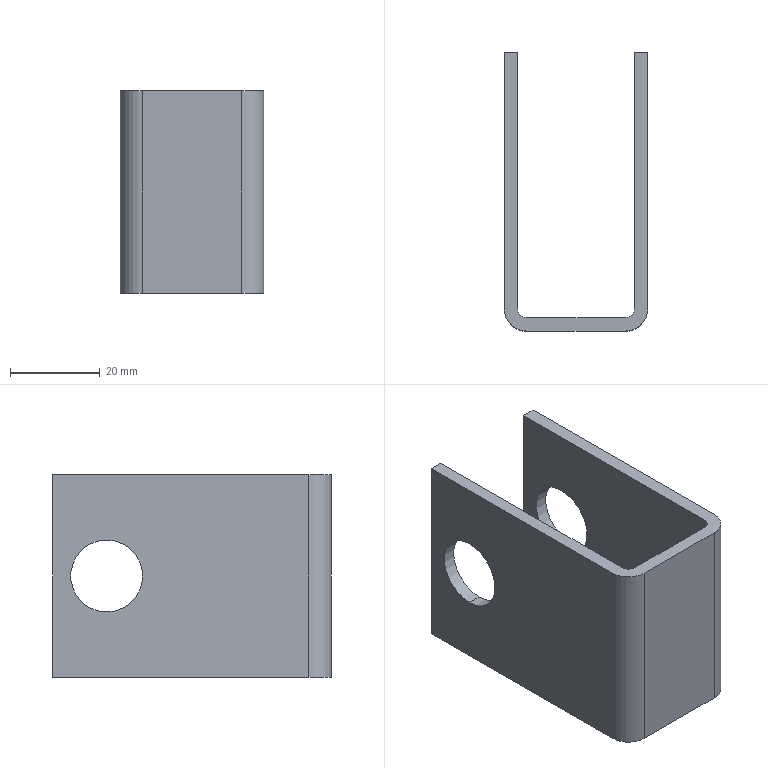Part | SolidWorks | features Extrusion 1, ICE 1 | 1 solid | 18 faces | box 32 x 62 x 45 mm | volume 18638 mm3 | plane 10 | cylinder 8 | commonest cylinder face diameters 16 x4 4 x2 10 x2
STEP:
#1=CARTESIAN_POINT('',(29.,-12.,30.5));
#2=VERTEX_POINT('',#1);
#3=CARTESIAN_POINT('',(29.,-12.,14.5));
#4=VERTEX_POINT('',#3);
#5=CARTESIAN_POINT('',(29.,-12.,22.5));
#6=DIRECTION('',(1.,0.,0.));
#7=DIRECTION('',(0.,1.,0.));
#8=AXIS2_PLACEMENT_3D('',#5,#6,#7);
#9=CIRCLE('',#8,8.);
#10=EDGE_CURVE('',#2,#4,#9,.T.);
#11=ORIENTED_EDGE('',*,*,#10,.F.);
#12=CARTESIAN_POINT('',(32.,-12.,30.5));
#13=VERTEX_POINT('',#12);
#14=CARTESIAN_POINT('',(0.,-12.,30.5));
#15=DIRECTION('',(1.,0.,0.));
#16=VECTOR('',#15,1000.);
#17=LINE('',#14,#16);
#18=EDGE_CURVE('',#2,#13,#17,.T.);
#19=ORIENTED_EDGE('',*,*,#18,.T.);
#20=CARTESIAN_POINT('',(32.,-12.,14.5));
#21=VERTEX_POINT('',#20);
#22=CARTESIAN_POINT('',(32.,-12.,22.5));
#23=DIRECTION('',(1.,0.,0.));
#24=DIRECTION('',(0.,0.,-1.));
#25=AXIS2_PLACEMENT_3D('',#22,#23,#24);
#26=CIRCLE('',#25,8.);
#27=EDGE_CURVE('',#13,#21,#26,.T.);
#28=ORIENTED_EDGE('',*,*,#27,.T.);
#29=CARTESIAN_POINT('',(0.,-12.,14.5));
#30=DIRECTION('',(1.,0.,0.));
#31=VECTOR('',#30,1000.);
#32=LINE('',#29,#31);
#33=EDGE_CURVE('',#4,#21,#32,.T.);
#34=ORIENTED_EDGE('',*,*,#33,.F.);
#35=EDGE_LOOP('',(#11,#19,#28,#34));
#36=FACE_OUTER_BOUND('',#35,.T.);
#37=CARTESIAN_POINT('',(0.,-12.,22.5));
#38=DIRECTION('',(1.,0.,0.));
#39=DIRECTION('',(0.,0.,-1.));
#40=AXIS2_PLACEMENT_3D('',#37,#38,#39);
#41=CYLINDRICAL_SURFACE('',#40,8.);
#42=ADVANCED_FACE('',(#36),#41,.F.);
#43=CARTESIAN_POINT('',(0.,-12.,30.5));
#44=VERTEX_POINT('',#43);
#45=CARTESIAN_POINT('',(0.,-12.,14.5));
#46=VERTEX_POINT('',#45);
#47=CARTESIAN_POINT('',(0.,-12.,22.5));
#48=DIRECTION('',(1.,0.,0.));
#49=DIRECTION('',(0.,0.,-1.));
#50=AXIS2_PLACEMENT_3D('',#47,#48,#49);
#51=CIRCLE('',#50,8.);
#52=EDGE_CURVE('',#44,#46,#51,.T.);
#53=ORIENTED_EDGE('',*,*,#52,.F.);
#54=CARTESIAN_POINT('',(3.,-12.,30.5));
#55=VERTEX_POINT('',#54);
#56=CARTESIAN_POINT('',(0.,-12.,30.5));
#57=DIRECTION('',(1.,0.,0.));
#58=VECTOR('',#57,1000.);
#59=LINE('',#56,#58);
#60=EDGE_CURVE('',#44,#55,#59,.T.);
#61=ORIENTED_EDGE('',*,*,#60,.T.);
#62=CARTESIAN_POINT('',(3.,-12.,14.5));
#63=VERTEX_POINT('',#62);
#64=CARTESIAN_POINT('',(3.,-12.,22.5));
#65=DIRECTION('',(-1.,0.,0.));
#66=DIRECTION('',(0.,0.,1.));
#67=AXIS2_PLACEMENT_3D('',#64,#65,#66);
#68=CIRCLE('',#67,8.);
#69=EDGE_CURVE('',#63,#55,#68,.T.);
#70=ORIENTED_EDGE('',*,*,#69,.F.);
#71=CARTESIAN_POINT('',(0.,-12.,14.5));
#72=DIRECTION('',(1.,0.,0.));
#73=VECTOR('',#72,1000.);
#74=LINE('',#71,#73);
#75=EDGE_CURVE('',#46,#63,#74,.T.);
#76=ORIENTED_EDGE('',*,*,#75,.F.);
#77=EDGE_LOOP('',(#53,#61,#70,#76));
#78=FACE_OUTER_BOUND('',#77,.T.);
#79=CARTESIAN_POINT('',(0.,-12.,22.5));
#80=DIRECTION('',(1.,0.,0.));
#81=DIRECTION('',(0.,0.,-1.));
#82=AXIS2_PLACEMENT_3D('',#79,#80,#81);
#83=CYLINDRICAL_SURFACE('',#82,8.);
#84=ADVANCED_FACE('',(#78),#83,.F.);
#85=CARTESIAN_POINT('',(3.,0.,0.));
#86=VERTEX_POINT('',#85);
#87=CARTESIAN_POINT('',(0.,0.,0.));
#88=VERTEX_POINT('',#87);
#89=CARTESIAN_POINT('',(3.,0.,0.));
#90=DIRECTION('',(-1.,0.,0.));
#91=VECTOR('',#90,1000.);
#92=LINE('',#89,#91);
#93=EDGE_CURVE('',#86,#88,#92,.T.);
#94=ORIENTED_EDGE('',*,*,#93,.T.);
#95=CARTESIAN_POINT('',(0.,0.,45.));
#96=VERTEX_POINT('',#95);
#97=CARTESIAN_POINT('',(0.,0.,45.));
#98=DIRECTION('',(0.,0.,-1.));
#99=VECTOR('',#98,1000.);
#100=LINE('',#97,#99);
#101=EDGE_CURVE('',#96,#88,#100,.T.);
#102=ORIENTED_EDGE('',*,*,#101,.F.);
#103=CARTESIAN_POINT('',(3.,0.,45.));
#104=VERTEX_POINT('',#103);
#105=CARTESIAN_POINT('',(3.,0.,45.));
#106=DIRECTION('',(-1.,0.,0.));
#107=VECTOR('',#106,1000.);
#108=LINE('',#105,#107);
#109=EDGE_CURVE('',#104,#96,#108,.T.);
#110=ORIENTED_EDGE('',*,*,#109,.F.);
#111=CARTESIAN_POINT('',(3.,0.,45.));
#112=DIRECTION('',(0.,0.,-1.));
#113=VECTOR('',#112,1000.);
#114=LINE('',#111,#113);
#115=EDGE_CURVE('',#104,#86,#114,.T.);
#116=ORIENTED_EDGE('',*,*,#115,.T.);
#117=EDGE_LOOP('',(#94,#102,#110,#116));
#118=FACE_OUTER_BOUND('',#117,.T.);
#119=CARTESIAN_POINT('',(3.,0.,45.));
#120=DIRECTION('',(0.,-1.,0.));
#121=DIRECTION('',(0.,0.,-1.));
#122=AXIS2_PLACEMENT_3D('',#119,#120,#121);
#123=PLANE('',#122);
#124=ADVANCED_FACE('',(#118),#123,.F.);
#125=CARTESIAN_POINT('',(0.,-12.,22.5));
#126=DIRECTION('',(1.,0.,0.));
#127=DIRECTION('',(0.,0.,-1.));
#128=AXIS2_PLACEMENT_3D('',#125,#126,#127);
#129=CIRCLE('',#128,8.);
#130=EDGE_CURVE('',#46,#44,#129,.T.);
#131=ORIENTED_EDGE('',*,*,#130,.T.);
#132=ORIENTED_EDGE('',*,*,#52,.T.);
#133=EDGE_LOOP('',(#131,#132));
#134=FACE_BOUND('',#133,.T.);
#135=CARTESIAN_POINT('',(0.,-57.,0.));
#136=VERTEX_POINT('',#135);
#137=CARTESIAN_POINT('',(0.,0.,0.));
#138=DIRECTION('',(0.,-1.,0.));
#139=VECTOR('',#138,1000.);
#140=LINE('',#137,#139);
#141=EDGE_CURVE('',#88,#136,#140,.T.);
#142=ORIENTED_EDGE('',*,*,#141,.T.);
#143=CARTESIAN_POINT('',(0.,-57.,45.));
#144=VERTEX_POINT('',#143);
#145=CARTESIAN_POINT('',(0.,-57.,45.));
#146=DIRECTION('',(0.,0.,-1.));
#147=VECTOR('',#146,1000.);
#148=LINE('',#145,#147);
#149=EDGE_CURVE('',#144,#136,#148,.T.);
#150=ORIENTED_EDGE('',*,*,#149,.F.);
#151=CARTESIAN_POINT('',(0.,0.,45.));
#152=DIRECTION('',(0.,-1.,0.));
#153=VECTOR('',#152,1000.);
#154=LINE('',#151,#153);
#155=EDGE_CURVE('',#96,#144,#154,.T.);
#156=ORIENTED_EDGE('',*,*,#155,.F.);
#157=ORIENTED_EDGE('',*,*,#101,.T.);
#158=EDGE_LOOP('',(#142,#150,#156,#157));
#159=FACE_OUTER_BOUND('',#158,.T.);
#160=CARTESIAN_POINT('',(0.,0.,45.));
#161=DIRECTION('',(1.,0.,0.));
#162=DIRECTION('',(0.,1.,0.));
#163=AXIS2_PLACEMENT_3D('',#160,#161,#162);
#164=PLANE('',#163);
#165=ADVANCED_FACE('',(#134,#159),#164,.F.);
#166=CARTESIAN_POINT('',(5.,-62.,0.));
#167=VERTEX_POINT('',#166);
#168=CARTESIAN_POINT('',(5.,-57.,0.));
#169=DIRECTION('',(0.,0.,1.));
#170=DIRECTION('',(1.,0.,0.));
#171=AXIS2_PLACEMENT_3D('',#168,#169,#170);
#172=CIRCLE('',#171,5.);
#173=EDGE_CURVE('',#136,#167,#172,.T.);
#174=ORIENTED_EDGE('',*,*,#173,.T.);
#175=CARTESIAN_POINT('',(5.,-62.,45.));
#176=VERTEX_POINT('',#175);
#177=CARTESIAN_POINT('',(5.,-62.,45.));
#178=DIRECTION('',(0.,0.,-1.));
#179=VECTOR('',#178,1000.);
#180=LINE('',#177,#179);
#181=EDGE_CURVE('',#176,#167,#180,.T.);
#182=ORIENTED_EDGE('',*,*,#181,.F.);
#183=CARTESIAN_POINT('',(5.,-57.,45.));
#184=DIRECTION('',(0.,0.,1.));
#185=DIRECTION('',(1.,0.,0.));
#186=AXIS2_PLACEMENT_3D('',#183,#184,#185);
#187=CIRCLE('',#186,5.);
#188=EDGE_CURVE('',#144,#176,#187,.T.);
#189=ORIENTED_EDGE('',*,*,#188,.F.);
#190=ORIENTED_EDGE('',*,*,#149,.T.);
#191=EDGE_LOOP('',(#174,#182,#189,#190));
#192=FACE_OUTER_BOUND('',#191,.T.);
#193=CARTESIAN_POINT('',(5.,-57.,45.));
#194=DIRECTION('',(0.,0.,-1.));
#195=DIRECTION('',(-1.,0.,0.));
#196=AXIS2_PLACEMENT_3D('',#193,#194,#195);
#197=CYLINDRICAL_SURFACE('',#196,5.);
#198=ADVANCED_FACE('',(#192),#197,.T.);
#199=CARTESIAN_POINT('',(27.,-62.,0.));
#200=VERTEX_POINT('',#199);
#201=CARTESIAN_POINT('',(5.,-62.,0.));
#202=DIRECTION('',(1.,0.,0.));
#203=VECTOR('',#202,1000.);
#204=LINE('',#201,#203);
#205=EDGE_CURVE('',#167,#200,#204,.T.);
#206=ORIENTED_EDGE('',*,*,#205,.T.);
#207=CARTESIAN_POINT('',(27.,-62.,45.));
#208=VERTEX_POINT('',#207);
#209=CARTESIAN_POINT('',(27.,-62.,45.));
#210=DIRECTION('',(0.,0.,-1.));
#211=VECTOR('',#210,1000.);
#212=LINE('',#209,#211);
#213=EDGE_CURVE('',#208,#200,#212,.T.);
#214=ORIENTED_EDGE('',*,*,#213,.F.);
#215=CARTESIAN_POINT('',(5.,-62.,45.));
#216=DIRECTION('',(1.,0.,0.));
#217=VECTOR('',#216,1000.);
#218=LINE('',#215,#217);
#219=EDGE_CURVE('',#176,#208,#218,.T.);
#220=ORIENTED_EDGE('',*,*,#219,.F.);
#221=ORIENTED_EDGE('',*,*,#181,.T.);
#222=EDGE_LOOP('',(#206,#214,#220,#221));
#223=FACE_OUTER_BOUND('',#222,.T.);
#224=CARTESIAN_POINT('',(5.,-62.,45.));
#225=DIRECTION('',(0.,1.,0.));
#226=DIRECTION('',(0.,0.,1.));
#227=AXIS2_PLACEMENT_3D('',#224,#225,#226);
#228=PLANE('',#227);
#229=ADVANCED_FACE('',(#223),#228,.F.);
#230=CARTESIAN_POINT('',(32.,-57.,0.));
#231=VERTEX_POINT('',#230);
#232=CARTESIAN_POINT('',(27.,-57.,0.));
#233=DIRECTION('',(0.,0.,1.));
#234=DIRECTION('',(1.,0.,0.));
#235=AXIS2_PLACEMENT_3D('',#232,#233,#234);
#236=CIRCLE('',#235,5.);
#237=EDGE_CURVE('',#200,#231,#236,.T.);
#238=ORIENTED_EDGE('',*,*,#237,.T.);
#239=CARTESIAN_POINT('',(32.,-57.,45.));
#240=VERTEX_POINT('',#239);
#241=CARTESIAN_POINT('',(32.,-57.,45.));
#242=DIRECTION('',(0.,0.,-1.));
#243=VECTOR('',#242,1000.);
#244=LINE('',#241,#243);
#245=EDGE_CURVE('',#240,#231,#244,.T.);
#246=ORIENTED_EDGE('',*,*,#245,.F.);
#247=CARTESIAN_POINT('',(27.,-57.,45.));
#248=DIRECTION('',(0.,0.,1.));
#249=DIRECTION('',(1.,0.,0.));
#250=AXIS2_PLACEMENT_3D('',#247,#248,#249);
#251=CIRCLE('',#250,5.);
#252=EDGE_CURVE('',#208,#240,#251,.T.);
#253=ORIENTED_EDGE('',*,*,#252,.F.);
#254=ORIENTED_EDGE('',*,*,#213,.T.);
#255=EDGE_LOOP('',(#238,#246,#253,#254));
#256=FACE_OUTER_BOUND('',#255,.T.);
#257=CARTESIAN_POINT('',(27.,-57.,45.));
#258=DIRECTION('',(0.,0.,-1.));
#259=DIRECTION('',(-1.,0.,0.));
#260=AXIS2_PLACEMENT_3D('',#257,#258,#259);
#261=CYLINDRICAL_SURFACE('',#260,5.);
#262=ADVANCED_FACE('',(#256),#261,.T.);
#263=CARTESIAN_POINT('',(32.,-12.,22.5));
#264=DIRECTION('',(1.,0.,0.));
#265=DIRECTION('',(0.,0.,-1.));
#266=AXIS2_PLACEMENT_3D('',#263,#264,#265);
#267=CIRCLE('',#266,8.);
#268=EDGE_CURVE('',#21,#13,#267,.T.);
#269=ORIENTED_EDGE('',*,*,#268,.F.);
#270=ORIENTED_EDGE('',*,*,#27,.F.);
#271=EDGE_LOOP('',(#269,#270));
#272=FACE_BOUND('',#271,.T.);
#273=CARTESIAN_POINT('',(32.,0.,0.));
#274=VERTEX_POINT('',#273);
#275=CARTESIAN_POINT('',(32.,-57.,0.));
#276=DIRECTION('',(0.,1.,0.));
#277=VECTOR('',#276,1000.);
#278=LINE('',#275,#277);
#279=EDGE_CURVE('',#231,#274,#278,.T.);
#280=ORIENTED_EDGE('',*,*,#279,.T.);
#281=CARTESIAN_POINT('',(32.,0.,45.));
#282=VERTEX_POINT('',#281);
#283=CARTESIAN_POINT('',(32.,0.,45.));
#284=DIRECTION('',(0.,0.,-1.));
#285=VECTOR('',#284,1000.);
#286=LINE('',#283,#285);
#287=EDGE_CURVE('',#282,#274,#286,.T.);
#288=ORIENTED_EDGE('',*,*,#287,.F.);
#289=CARTESIAN_POINT('',(32.,-57.,45.));
#290=DIRECTION('',(0.,1.,0.));
#291=VECTOR('',#290,1000.);
#292=LINE('',#289,#291);
#293=EDGE_CURVE('',#240,#282,#292,.T.);
#294=ORIENTED_EDGE('',*,*,#293,.F.);
#295=ORIENTED_EDGE('',*,*,#245,.T.);
#296=EDGE_LOOP('',(#280,#288,#294,#295));
#297=FACE_OUTER_BOUND('',#296,.T.);
#298=CARTESIAN_POINT('',(32.,-57.,45.));
#299=DIRECTION('',(-1.,0.,0.));
#300=DIRECTION('',(0.,0.,1.));
#301=AXIS2_PLACEMENT_3D('',#298,#299,#300);
#302=PLANE('',#301);
#303=ADVANCED_FACE('',(#272,#297),#302,.F.);
#304=CARTESIAN_POINT('',(29.,0.,0.));
#305=VERTEX_POINT('',#304);
#306=CARTESIAN_POINT('',(29.,0.,0.));
#307=DIRECTION('',(-1.,0.,0.));
#308=VECTOR('',#307,1000.);
#309=LINE('',#306,#308);
#310=EDGE_CURVE('',#274,#305,#309,.T.);
#311=ORIENTED_EDGE('',*,*,#310,.T.);
#312=CARTESIAN_POINT('',(29.,0.,45.));
#313=VERTEX_POINT('',#312);
#314=CARTESIAN_POINT('',(29.,0.,45.));
#315=DIRECTION('',(0.,0.,-1.));
#316=VECTOR('',#315,1000.);
#317=LINE('',#314,#316);
#318=EDGE_CURVE('',#313,#305,#317,.T.);
#319=ORIENTED_EDGE('',*,*,#318,.F.);
#320=CARTESIAN_POINT('',(29.,0.,45.));
#321=DIRECTION('',(-1.,0.,0.));
#322=VECTOR('',#321,1000.);
#323=LINE('',#320,#322);
#324=EDGE_CURVE('',#282,#313,#323,.T.);
#325=ORIENTED_EDGE('',*,*,#324,.F.);
#326=ORIENTED_EDGE('',*,*,#287,.T.);
#327=EDGE_LOOP('',(#311,#319,#325,#326));
#328=FACE_OUTER_BOUND('',#327,.T.);
#329=CARTESIAN_POINT('',(29.,0.,45.));
#330=DIRECTION('',(0.,-1.,0.));
#331=DIRECTION('',(0.,0.,-1.));
#332=AXIS2_PLACEMENT_3D('',#329,#330,#331);
#333=PLANE('',#332);
#334=ADVANCED_FACE('',(#328),#333,.F.);
#335=CARTESIAN_POINT('',(29.,-12.,22.5));
#336=DIRECTION('',(1.,0.,0.));
#337=DIRECTION('',(0.,1.,0.));
#338=AXIS2_PLACEMENT_3D('',#335,#336,#337);
#339=CIRCLE('',#338,8.);
#340=EDGE_CURVE('',#4,#2,#339,.T.);
#341=ORIENTED_EDGE('',*,*,#340,.T.);
#342=ORIENTED_EDGE('',*,*,#10,.T.);
#343=EDGE_LOOP('',(#341,#342));
#344=FACE_BOUND('',#343,.T.);
#345=CARTESIAN_POINT('',(29.,-57.,0.));
#346=VERTEX_POINT('',#345);
#347=CARTESIAN_POINT('',(29.,-57.,0.));
#348=DIRECTION('',(0.,-1.,0.));
#349=VECTOR('',#348,1000.);
#350=LINE('',#347,#349);
#351=EDGE_CURVE('',#305,#346,#350,.T.);
#352=ORIENTED_EDGE('',*,*,#351,.T.);
#353=CARTESIAN_POINT('',(29.,-57.,45.));
#354=VERTEX_POINT('',#353);
#355=CARTESIAN_POINT('',(29.,-57.,45.));
#356=DIRECTION('',(0.,0.,-1.));
#357=VECTOR('',#356,1000.);
#358=LINE('',#355,#357);
#359=EDGE_CURVE('',#354,#346,#358,.T.);
#360=ORIENTED_EDGE('',*,*,#359,.F.);
#361=CARTESIAN_POINT('',(29.,-57.,45.));
#362=DIRECTION('',(0.,-1.,0.));
#363=VECTOR('',#362,1000.);
#364=LINE('',#361,#363);
#365=EDGE_CURVE('',#313,#354,#364,.T.);
#366=ORIENTED_EDGE('',*,*,#365,.F.);
#367=ORIENTED_EDGE('',*,*,#318,.T.);
#368=EDGE_LOOP('',(#352,#360,#366,#367));
#369=FACE_OUTER_BOUND('',#368,.T.);
#370=CARTESIAN_POINT('',(29.,-57.,45.));
#371=DIRECTION('',(1.,0.,0.));
#372=DIRECTION('',(0.,1.,0.));
#373=AXIS2_PLACEMENT_3D('',#370,#371,#372);
#374=PLANE('',#373);
#375=ADVANCED_FACE('',(#344,#369),#374,.F.);
#376=CARTESIAN_POINT('',(27.,-59.,0.));
#377=VERTEX_POINT('',#376);
#378=CARTESIAN_POINT('',(27.,-57.,0.));
#379=DIRECTION('',(0.,0.,-1.));
#380=DIRECTION('',(1.,0.,0.));
#381=AXIS2_PLACEMENT_3D('',#378,#379,#380);
#382=CIRCLE('',#381,2.);
#383=EDGE_CURVE('',#346,#377,#382,.T.);
#384=ORIENTED_EDGE('',*,*,#383,.T.);
#385=CARTESIAN_POINT('',(27.,-59.,45.));
#386=VERTEX_POINT('',#385);
#387=CARTESIAN_POINT('',(27.,-59.,45.));
#388=DIRECTION('',(0.,0.,-1.));
#389=VECTOR('',#388,1000.);
#390=LINE('',#387,#389);
#391=EDGE_CURVE('',#386,#377,#390,.T.);
#392=ORIENTED_EDGE('',*,*,#391,.F.);
#393=CARTESIAN_POINT('',(27.,-57.,45.));
#394=DIRECTION('',(0.,0.,-1.));
#395=DIRECTION('',(1.,0.,0.));
#396=AXIS2_PLACEMENT_3D('',#393,#394,#395);
#397=CIRCLE('',#396,2.);
#398=EDGE_CURVE('',#354,#386,#397,.T.);
#399=ORIENTED_EDGE('',*,*,#398,.F.);
#400=ORIENTED_EDGE('',*,*,#359,.T.);
#401=EDGE_LOOP('',(#384,#392,#399,#400));
#402=FACE_OUTER_BOUND('',#401,.T.);
#403=CARTESIAN_POINT('',(27.,-57.,45.));
#404=DIRECTION('',(0.,0.,-1.));
#405=DIRECTION('',(-1.,0.,0.));
#406=AXIS2_PLACEMENT_3D('',#403,#404,#405);
#407=CYLINDRICAL_SURFACE('',#406,2.);
#408=ADVANCED_FACE('',(#402),#407,.F.);
#409=CARTESIAN_POINT('',(5.,-59.,0.));
#410=VERTEX_POINT('',#409);
#411=CARTESIAN_POINT('',(5.,-59.,0.));
#412=DIRECTION('',(-1.,0.,0.));
#413=VECTOR('',#412,1000.);
#414=LINE('',#411,#413);
#415=EDGE_CURVE('',#377,#410,#414,.T.);
#416=ORIENTED_EDGE('',*,*,#415,.T.);
#417=CARTESIAN_POINT('',(5.,-59.,45.));
#418=VERTEX_POINT('',#417);
#419=CARTESIAN_POINT('',(5.,-59.,45.));
#420=DIRECTION('',(0.,0.,-1.));
#421=VECTOR('',#420,1000.);
#422=LINE('',#419,#421);
#423=EDGE_CURVE('',#418,#410,#422,.T.);
#424=ORIENTED_EDGE('',*,*,#423,.F.);
#425=CARTESIAN_POINT('',(5.,-59.,45.));
#426=DIRECTION('',(-1.,0.,0.));
#427=VECTOR('',#426,1000.);
#428=LINE('',#425,#427);
#429=EDGE_CURVE('',#386,#418,#428,.T.);
#430=ORIENTED_EDGE('',*,*,#429,.F.);
#431=ORIENTED_EDGE('',*,*,#391,.T.);
#432=EDGE_LOOP('',(#416,#424,#430,#431));
#433=FACE_OUTER_BOUND('',#432,.T.);
#434=CARTESIAN_POINT('',(5.,-59.,45.));
#435=DIRECTION('',(0.,-1.,0.));
#436=DIRECTION('',(0.,0.,-1.));
#437=AXIS2_PLACEMENT_3D('',#434,#435,#436);
#438=PLANE('',#437);
#439=ADVANCED_FACE('',(#433),#438,.F.);
#440=CARTESIAN_POINT('',(3.,-57.,0.));
#441=VERTEX_POINT('',#440);
#442=CARTESIAN_POINT('',(5.,-57.,0.));
#443=DIRECTION('',(0.,0.,-1.));
#444=DIRECTION('',(1.,0.,0.));
#445=AXIS2_PLACEMENT_3D('',#442,#443,#444);
#446=CIRCLE('',#445,2.);
#447=EDGE_CURVE('',#410,#441,#446,.T.);
#448=ORIENTED_EDGE('',*,*,#447,.T.);
#449=CARTESIAN_POINT('',(3.,-57.,45.));
#450=VERTEX_POINT('',#449);
#451=CARTESIAN_POINT('',(3.,-57.,45.));
#452=DIRECTION('',(0.,0.,-1.));
#453=VECTOR('',#452,1000.);
#454=LINE('',#451,#453);
#455=EDGE_CURVE('',#450,#441,#454,.T.);
#456=ORIENTED_EDGE('',*,*,#455,.F.);
#457=CARTESIAN_POINT('',(5.,-57.,45.));
#458=DIRECTION('',(0.,0.,-1.));
#459=DIRECTION('',(1.,0.,0.));
#460=AXIS2_PLACEMENT_3D('',#457,#458,#459);
#461=CIRCLE('',#460,2.);
#462=EDGE_CURVE('',#418,#450,#461,.T.);
#463=ORIENTED_EDGE('',*,*,#462,.F.);
#464=ORIENTED_EDGE('',*,*,#423,.T.);
#465=EDGE_LOOP('',(#448,#456,#463,#464));
#466=FACE_OUTER_BOUND('',#465,.T.);
#467=CARTESIAN_POINT('',(5.,-57.,45.));
#468=DIRECTION('',(0.,0.,-1.));
#469=DIRECTION('',(-1.,0.,0.));
#470=AXIS2_PLACEMENT_3D('',#467,#468,#469);
#471=CYLINDRICAL_SURFACE('',#470,2.);
#472=ADVANCED_FACE('',(#466),#471,.F.);
#473=ORIENTED_EDGE('',*,*,#69,.T.);
#474=CARTESIAN_POINT('',(3.,-12.,22.5));
#475=DIRECTION('',(-1.,0.,0.));
#476=DIRECTION('',(0.,0.,1.));
#477=AXIS2_PLACEMENT_3D('',#474,#475,#476);
#478=CIRCLE('',#477,8.);
#479=EDGE_CURVE('',#55,#63,#478,.T.);
#480=ORIENTED_EDGE('',*,*,#479,.T.);
#481=EDGE_LOOP('',(#473,#480));
#482=FACE_BOUND('',#481,.T.);
#483=CARTESIAN_POINT('',(3.,0.,0.));
#484=DIRECTION('',(0.,1.,0.));
#485=VECTOR('',#484,1000.);
#486=LINE('',#483,#485);
#487=EDGE_CURVE('',#441,#86,#486,.T.);
#488=ORIENTED_EDGE('',*,*,#487,.T.);
#489=ORIENTED_EDGE('',*,*,#115,.F.);
#490=CARTESIAN_POINT('',(3.,0.,45.));
#491=DIRECTION('',(0.,1.,0.));
#492=VECTOR('',#491,1000.);
#493=LINE('',#490,#492);
#494=EDGE_CURVE('',#450,#104,#493,.T.);
#495=ORIENTED_EDGE('',*,*,#494,.F.);
#496=ORIENTED_EDGE('',*,*,#455,.T.);
#497=EDGE_LOOP('',(#488,#489,#495,#496));
#498=FACE_OUTER_BOUND('',#497,.T.);
#499=CARTESIAN_POINT('',(3.,0.,45.));
#500=DIRECTION('',(-1.,0.,0.));
#501=DIRECTION('',(0.,0.,1.));
#502=AXIS2_PLACEMENT_3D('',#499,#500,#501);
#503=PLANE('',#502);
#504=ADVANCED_FACE('',(#482,#498),#503,.F.);
#505=ORIENTED_EDGE('',*,*,#109,.T.);
#506=ORIENTED_EDGE('',*,*,#155,.T.);
#507=ORIENTED_EDGE('',*,*,#188,.T.);
#508=ORIENTED_EDGE('',*,*,#219,.T.);
#509=ORIENTED_EDGE('',*,*,#252,.T.);
#510=ORIENTED_EDGE('',*,*,#293,.T.);
#511=ORIENTED_EDGE('',*,*,#324,.T.);
#512=ORIENTED_EDGE('',*,*,#365,.T.);
#513=ORIENTED_EDGE('',*,*,#398,.T.);
#514=ORIENTED_EDGE('',*,*,#429,.T.);
#515=ORIENTED_EDGE('',*,*,#462,.T.);
#516=ORIENTED_EDGE('',*,*,#494,.T.);
#517=EDGE_LOOP('',(#505,#506,#507,#508,#509,#510,#511,#512,#513,#514,#515,#516));
#518=FACE_OUTER_BOUND('',#517,.T.);
#519=CARTESIAN_POINT('',(5.,-57.,45.));
#520=DIRECTION('',(0.,0.,1.));
#521=DIRECTION('',(1.,0.,0.));
#522=AXIS2_PLACEMENT_3D('',#519,#520,#521);
#523=PLANE('',#522);
#524=ADVANCED_FACE('',(#518),#523,.T.);
#525=ORIENTED_EDGE('',*,*,#93,.F.);
#526=ORIENTED_EDGE('',*,*,#487,.F.);
#527=ORIENTED_EDGE('',*,*,#447,.F.);
#528=ORIENTED_EDGE('',*,*,#415,.F.);
#529=ORIENTED_EDGE('',*,*,#383,.F.);
#530=ORIENTED_EDGE('',*,*,#351,.F.);
#531=ORIENTED_EDGE('',*,*,#310,.F.);
#532=ORIENTED_EDGE('',*,*,#279,.F.);
#533=ORIENTED_EDGE('',*,*,#237,.F.);
#534=ORIENTED_EDGE('',*,*,#205,.F.);
#535=ORIENTED_EDGE('',*,*,#173,.F.);
#536=ORIENTED_EDGE('',*,*,#141,.F.);
#537=EDGE_LOOP('',(#525,#526,#527,#528,#529,#530,#531,#532,#533,#534,#535,#536));
#538=FACE_OUTER_BOUND('',#537,.T.);
#539=CARTESIAN_POINT('',(5.,-57.,0.));
#540=DIRECTION('',(0.,0.,1.));
#541=DIRECTION('',(1.,0.,0.));
#542=AXIS2_PLACEMENT_3D('',#539,#540,#541);
#543=PLANE('',#542);
#544=ADVANCED_FACE('',(#538),#543,.F.);
#545=ORIENTED_EDGE('',*,*,#60,.F.);
#546=ORIENTED_EDGE('',*,*,#130,.F.);
#547=ORIENTED_EDGE('',*,*,#75,.T.);
#548=ORIENTED_EDGE('',*,*,#479,.F.);
#549=EDGE_LOOP('',(#545,#546,#547,#548));
#550=FACE_OUTER_BOUND('',#549,.T.);
#551=CARTESIAN_POINT('',(0.,-12.,22.5));
#552=DIRECTION('',(1.,0.,0.));
#553=DIRECTION('',(0.,0.,-1.));
#554=AXIS2_PLACEMENT_3D('',#551,#552,#553);
#555=CYLINDRICAL_SURFACE('',#554,8.);
#556=ADVANCED_FACE('',(#550),#555,.F.);
#557=ORIENTED_EDGE('',*,*,#18,.F.);
#558=ORIENTED_EDGE('',*,*,#340,.F.);
#559=ORIENTED_EDGE('',*,*,#33,.T.);
#560=ORIENTED_EDGE('',*,*,#268,.T.);
#561=EDGE_LOOP('',(#557,#558,#559,#560));
#562=FACE_OUTER_BOUND('',#561,.T.);
#563=CARTESIAN_POINT('',(0.,-12.,22.5));
#564=DIRECTION('',(1.,0.,0.));
#565=DIRECTION('',(0.,0.,-1.));
#566=AXIS2_PLACEMENT_3D('',#563,#564,#565);
#567=CYLINDRICAL_SURFACE('',#566,8.);
#568=ADVANCED_FACE('',(#562),#567,.F.);
#569=CLOSED_SHELL('',(#42,#84,#124,#165,#198,#229,#262,#303,#334,#375,#408,#439,#472,#504,#524,#544,#556,#568));
#570=MANIFOLD_SOLID_BREP('',#569);
#571=CARTESIAN_POINT('',(0.,0.,0.));
#572=DIRECTION('',(0.,0.,1.));
#573=DIRECTION('',(1.,0.,0.));
#574=AXIS2_PLACEMENT_3D('',#571,#572,#573);
#575=(LENGTH_UNIT()NAMED_UNIT(*)SI_UNIT(.MILLI.,.METRE.));
#576=UNCERTAINTY_MEASURE_WITH_UNIT(LENGTH_MEASURE(0.00001),#575,'','');
#577=(NAMED_UNIT(*)PLANE_ANGLE_UNIT()SI_UNIT($,.RADIAN.));
#578=(NAMED_UNIT(*)SI_UNIT($,.STERADIAN.)SOLID_ANGLE_UNIT());
#579=(GEOMETRIC_REPRESENTATION_CONTEXT(3)GLOBAL_UNCERTAINTY_ASSIGNED_CONTEXT((#576))GLOBAL_UNIT_ASSIGNED_CONTEXT((#575,#577,#578))REPRESENTATION_CONTEXT('',''));
#580=ADVANCED_BREP_SHAPE_REPRESENTATION('',(#570,#574),#579);